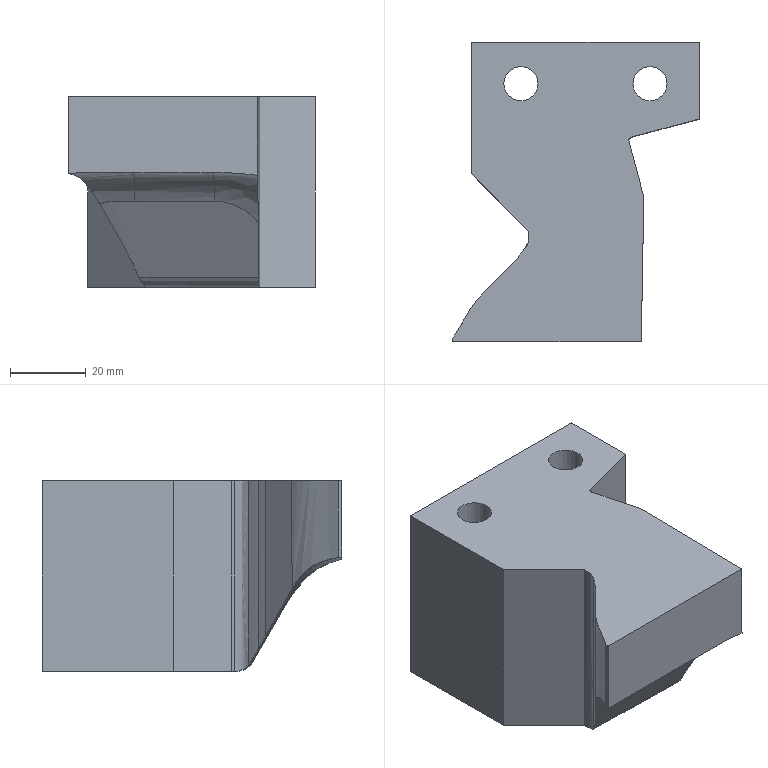Part | NX | features solid 2 | 1 solid | 34 faces | box 65 x 79 x 50.25 mm | volume 146603 mm3 | plane 17 | cylinder 11 | spline 5 | cone 1 | commonest cylinder face diameters 9.009 x2 10 x2 14.507 x2 2 x1 6.805 x1 7 x1